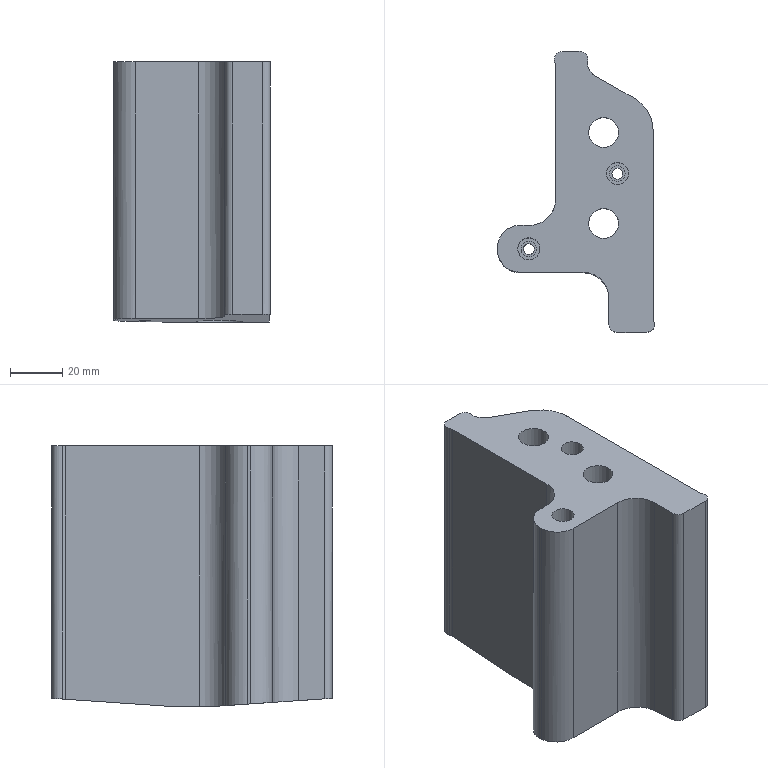Part | STEP file | lll_id266_x_t | 1 solid | 55 faces | box 60.307 x 107.85 x 100 mm | volume 310769 mm3 | cylinder 34 | plane 20 | cone 1 | commonest cylinder face diameters 6 x9 4.2 x2 8.5 x2 11.5 x2 17 x2 18.008 x2